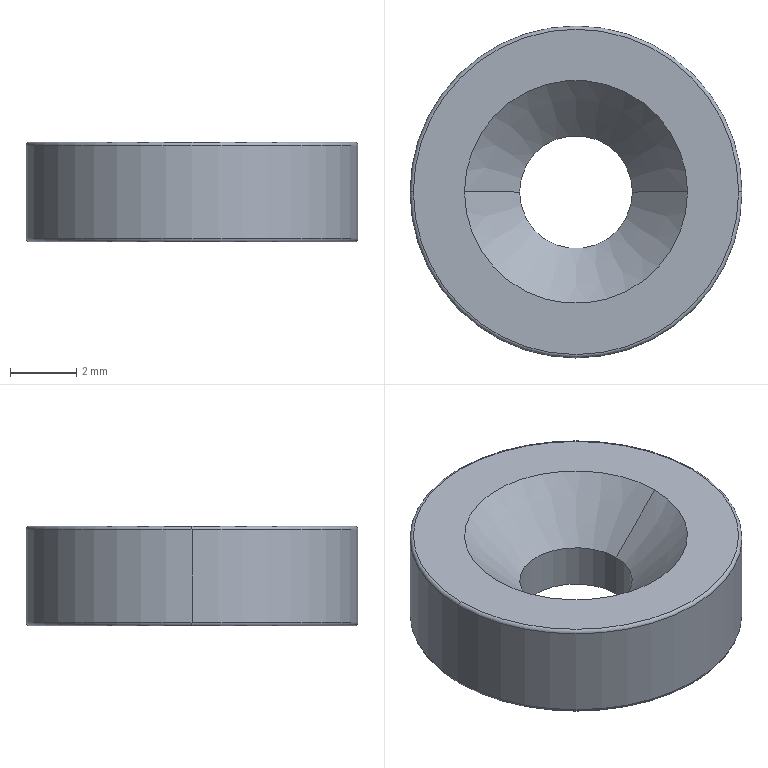Part | STEP file | QA-KZH10-3 | 1 solid | 12 faces | box 10 x 10 x 3 mm | volume 188.741 mm3 | torus 4 | cylinder 4 | cone 2 | plane 2 | commonest cylinder face diameters 3.4 x2 10 x2
STEP:
#1=CARTESIAN_POINT('',(0.,0.,0.));
#2=DIRECTION('',(0.,0.,1.));
#3=DIRECTION('',(1.,0.,0.));
#4=AXIS2_PLACEMENT_3D('',#1,#2,#3);
#5=CARTESIAN_POINT('',(-5.,0.,2.9));
#6=VERTEX_POINT('',#5);
#7=CARTESIAN_POINT('',(5.,0.,2.9));
#8=VERTEX_POINT('',#7);
#9=CARTESIAN_POINT('',(0.,0.,2.9));
#10=DIRECTION('',(0.,0.,-1.));
#11=DIRECTION('',(1.,0.,0.));
#12=AXIS2_PLACEMENT_3D('',#9,#10,#11);
#13=CIRCLE('',#12,5.);
#14=CARTESIAN_POINT('',(0.,0.,2.9));
#15=DIRECTION('',(0.,0.,1.));
#16=DIRECTION('',(1.,0.,0.));
#17=AXIS2_PLACEMENT_3D('',#14,#15,#16);
#18=TOROIDAL_SURFACE('',#17,4.9,0.1);
#19=CARTESIAN_POINT('',(6.283,0.));
#20=DIRECTION('',(-1.,0.));
#21=VECTOR('',#20,1.);
#22=LINE('',#19,#21);
#23=(GEOMETRIC_REPRESENTATION_CONTEXT(2)PARAMETRIC_REPRESENTATION_CONTEXT()REPRESENTATION_CONTEXT('',''));
#24=DEFINITIONAL_REPRESENTATION('',(#22),#23);
#25=PCURVE('',#18,#24);
#26=CARTESIAN_POINT('',(0.,0.,3.));
#27=DIRECTION('',(0.,0.,-1.));
#28=DIRECTION('',(-1.,0.,0.));
#29=AXIS2_PLACEMENT_3D('',#26,#27,#28);
#30=CYLINDRICAL_SURFACE('',#29,5.);
#31=CARTESIAN_POINT('',(-3.142,0.1));
#32=DIRECTION('',(1.,0.));
#33=VECTOR('',#32,1.);
#34=LINE('',#31,#33);
#35=(GEOMETRIC_REPRESENTATION_CONTEXT(2)PARAMETRIC_REPRESENTATION_CONTEXT()REPRESENTATION_CONTEXT('',''));
#36=DEFINITIONAL_REPRESENTATION('',(#34),#35);
#37=PCURVE('',#30,#36);
#38=SURFACE_CURVE('',#13,(#25,#37),.PCURVE_S1.);
#39=EDGE_CURVE('',#6,#8,#38,.T.);
#40=ORIENTED_EDGE('',*,*,#39,.F.);
#41=CARTESIAN_POINT('',(-4.9,0.,3.));
#42=VERTEX_POINT('',#41);
#43=CARTESIAN_POINT('',(-4.9,0.,2.9));
#44=DIRECTION('',(0.,1.,0.));
#45=DIRECTION('',(-1.,0.,0.));
#46=AXIS2_PLACEMENT_3D('',#43,#44,#45);
#47=CIRCLE('',#46,0.1);
#48=CARTESIAN_POINT('',(3.142,0.));
#49=DIRECTION('',(0.,1.));
#50=VECTOR('',#49,1.);
#51=LINE('',#48,#50);
#52=(GEOMETRIC_REPRESENTATION_CONTEXT(2)PARAMETRIC_REPRESENTATION_CONTEXT()REPRESENTATION_CONTEXT('',''));
#53=DEFINITIONAL_REPRESENTATION('',(#51),#52);
#54=PCURVE('',#18,#53);
#55=CARTESIAN_POINT('',(0.,0.,2.9));
#56=DIRECTION('',(0.,0.,1.));
#57=DIRECTION('',(1.,0.,0.));
#58=AXIS2_PLACEMENT_3D('',#55,#56,#57);
#59=TOROIDAL_SURFACE('',#58,4.9,0.1);
#60=CARTESIAN_POINT('',(3.142,0.));
#61=DIRECTION('',(0.,1.));
#62=VECTOR('',#61,1.);
#63=LINE('',#60,#62);
#64=(GEOMETRIC_REPRESENTATION_CONTEXT(2)PARAMETRIC_REPRESENTATION_CONTEXT()REPRESENTATION_CONTEXT('',''));
#65=DEFINITIONAL_REPRESENTATION('',(#63),#64);
#66=PCURVE('',#59,#65);
#67=SURFACE_CURVE('',#47,(#54,#66),.PCURVE_S1.);
#68=EDGE_CURVE('',#6,#42,#67,.T.);
#69=ORIENTED_EDGE('',*,*,#68,.T.);
#70=CARTESIAN_POINT('',(4.9,0.,3.));
#71=VERTEX_POINT('',#70);
#72=CARTESIAN_POINT('',(0.,0.,3.));
#73=DIRECTION('',(0.,0.,1.));
#74=DIRECTION('',(1.,0.,0.));
#75=AXIS2_PLACEMENT_3D('',#72,#73,#74);
#76=CIRCLE('',#75,4.9);
#77=CARTESIAN_POINT('',(0.,1.571));
#78=DIRECTION('',(1.,0.));
#79=VECTOR('',#78,1.);
#80=LINE('',#77,#79);
#81=(GEOMETRIC_REPRESENTATION_CONTEXT(2)PARAMETRIC_REPRESENTATION_CONTEXT()REPRESENTATION_CONTEXT('',''));
#82=DEFINITIONAL_REPRESENTATION('',(#80),#81);
#83=PCURVE('',#18,#82);
#84=CARTESIAN_POINT('',(0.,0.,3.));
#85=DIRECTION('',(0.,0.,1.));
#86=DIRECTION('',(1.,0.,0.));
#87=AXIS2_PLACEMENT_3D('',#84,#85,#86);
#88=PLANE('',#87);
#89=CARTESIAN_POINT('',(0.,0.));
#90=DIRECTION('',(1.,0.));
#91=AXIS2_PLACEMENT_2D('',#89,#90);
#92=CIRCLE('',#91,4.9);
#93=(GEOMETRIC_REPRESENTATION_CONTEXT(2)PARAMETRIC_REPRESENTATION_CONTEXT()REPRESENTATION_CONTEXT('',''));
#94=DEFINITIONAL_REPRESENTATION('',(#92),#93);
#95=PCURVE('',#88,#94);
#96=SURFACE_CURVE('',#76,(#83,#95),.PCURVE_S1.);
#97=EDGE_CURVE('',#71,#42,#96,.T.);
#98=ORIENTED_EDGE('',*,*,#97,.F.);
#99=CARTESIAN_POINT('',(4.9,0.,2.9));
#100=DIRECTION('',(0.,-1.,0.));
#101=DIRECTION('',(0.,0.,-1.));
#102=AXIS2_PLACEMENT_3D('',#99,#100,#101);
#103=CIRCLE('',#102,0.1);
#104=CARTESIAN_POINT('',(0.,-1.571));
#105=DIRECTION('',(0.,1.));
#106=VECTOR('',#105,1.);
#107=LINE('',#104,#106);
#108=(GEOMETRIC_REPRESENTATION_CONTEXT(2)PARAMETRIC_REPRESENTATION_CONTEXT()REPRESENTATION_CONTEXT('',''));
#109=DEFINITIONAL_REPRESENTATION('',(#107),#108);
#110=PCURVE('',#18,#109);
#111=CARTESIAN_POINT('',(6.283,-1.571));
#112=DIRECTION('',(0.,1.));
#113=VECTOR('',#112,1.);
#114=LINE('',#111,#113);
#115=(GEOMETRIC_REPRESENTATION_CONTEXT(2)PARAMETRIC_REPRESENTATION_CONTEXT()REPRESENTATION_CONTEXT('',''));
#116=DEFINITIONAL_REPRESENTATION('',(#114),#115);
#117=PCURVE('',#59,#116);
#118=SURFACE_CURVE('',#103,(#110,#117),.PCURVE_S1.);
#119=EDGE_CURVE('',#8,#71,#118,.T.);
#120=ORIENTED_EDGE('',*,*,#119,.F.);
#121=EDGE_LOOP('',(#40,#69,#98,#120));
#122=FACE_BOUND('',#121,.T.);
#123=ADVANCED_FACE('',(#122),#18,.T.);
#124=CARTESIAN_POINT('',(-4.9,0.,0.));
#125=VERTEX_POINT('',#124);
#126=CARTESIAN_POINT('',(4.9,0.,0.));
#127=VERTEX_POINT('',#126);
#128=CARTESIAN_POINT('',(0.,0.,0.));
#129=DIRECTION('',(0.,0.,-1.));
#130=DIRECTION('',(1.,0.,0.));
#131=AXIS2_PLACEMENT_3D('',#128,#129,#130);
#132=CIRCLE('',#131,4.9);
#133=CARTESIAN_POINT('',(0.,0.,0.1));
#134=DIRECTION('',(0.,0.,1.));
#135=DIRECTION('',(1.,0.,0.));
#136=AXIS2_PLACEMENT_3D('',#133,#134,#135);
#137=TOROIDAL_SURFACE('',#136,4.9,0.1);
#138=CARTESIAN_POINT('',(6.283,4.712));
#139=DIRECTION('',(-1.,0.));
#140=VECTOR('',#139,1.);
#141=LINE('',#138,#140);
#142=(GEOMETRIC_REPRESENTATION_CONTEXT(2)PARAMETRIC_REPRESENTATION_CONTEXT()REPRESENTATION_CONTEXT('',''));
#143=DEFINITIONAL_REPRESENTATION('',(#141),#142);
#144=PCURVE('',#137,#143);
#145=CARTESIAN_POINT('',(0.,0.,0.));
#146=DIRECTION('',(0.,0.,1.));
#147=DIRECTION('',(1.,0.,0.));
#148=AXIS2_PLACEMENT_3D('',#145,#146,#147);
#149=PLANE('',#148);
#150=CARTESIAN_POINT('',(4.9,0.));
#151=CARTESIAN_POINT('',(4.9,-8.487));
#152=CARTESIAN_POINT('',(-2.45,-4.244));
#153=CARTESIAN_POINT('',(-9.8,0.));
#154=CARTESIAN_POINT('',(-2.45,4.244));
#155=CARTESIAN_POINT('',(4.9,8.487));
#156=CARTESIAN_POINT('',(4.9,0.));
#157=(BOUNDED_CURVE()B_SPLINE_CURVE(2,(#150,#151,#152,#153,#154,#155,#156),.UNSPECIFIED.,.T.,.F.)B_SPLINE_CURVE_WITH_KNOTS((1,2,2,2,2,1),(-2.094,0.,2.094,4.189,6.283,8.378),.UNSPECIFIED.)CURVE()GEOMETRIC_REPRESENTATION_ITEM()RATIONAL_B_SPLINE_CURVE((1.,0.5,1.,0.5,1.,0.5,1.))REPRESENTATION_ITEM(''));
#158=(GEOMETRIC_REPRESENTATION_CONTEXT(2)PARAMETRIC_REPRESENTATION_CONTEXT()REPRESENTATION_CONTEXT('',''));
#159=DEFINITIONAL_REPRESENTATION('',(#157),#158);
#160=PCURVE('',#149,#159);
#161=SURFACE_CURVE('',#132,(#144,#160),.PCURVE_S1.);
#162=EDGE_CURVE('',#125,#127,#161,.T.);
#163=ORIENTED_EDGE('',*,*,#162,.F.);
#164=CARTESIAN_POINT('',(-5.,0.,0.1));
#165=VERTEX_POINT('',#164);
#166=CARTESIAN_POINT('',(-4.9,0.,0.1));
#167=DIRECTION('',(0.,1.,0.));
#168=DIRECTION('',(-1.,0.,0.));
#169=AXIS2_PLACEMENT_3D('',#166,#167,#168);
#170=CIRCLE('',#169,0.1);
#171=CARTESIAN_POINT('',(3.142,0.));
#172=DIRECTION('',(0.,1.));
#173=VECTOR('',#172,1.);
#174=LINE('',#171,#173);
#175=(GEOMETRIC_REPRESENTATION_CONTEXT(2)PARAMETRIC_REPRESENTATION_CONTEXT()REPRESENTATION_CONTEXT('',''));
#176=DEFINITIONAL_REPRESENTATION('',(#174),#175);
#177=PCURVE('',#137,#176);
#178=CARTESIAN_POINT('',(0.,0.,0.1));
#179=DIRECTION('',(0.,0.,1.));
#180=DIRECTION('',(1.,0.,0.));
#181=AXIS2_PLACEMENT_3D('',#178,#179,#180);
#182=TOROIDAL_SURFACE('',#181,4.9,0.1);
#183=CARTESIAN_POINT('',(3.142,0.));
#184=DIRECTION('',(0.,1.));
#185=VECTOR('',#184,1.);
#186=LINE('',#183,#185);
#187=(GEOMETRIC_REPRESENTATION_CONTEXT(2)PARAMETRIC_REPRESENTATION_CONTEXT()REPRESENTATION_CONTEXT('',''));
#188=DEFINITIONAL_REPRESENTATION('',(#186),#187);
#189=PCURVE('',#182,#188);
#190=SURFACE_CURVE('',#170,(#177,#189),.PCURVE_S1.);
#191=EDGE_CURVE('',#125,#165,#190,.T.);
#192=ORIENTED_EDGE('',*,*,#191,.T.);
#193=CARTESIAN_POINT('',(5.,0.,0.1));
#194=VERTEX_POINT('',#193);
#195=CARTESIAN_POINT('',(0.,0.,0.1));
#196=DIRECTION('',(0.,0.,1.));
#197=DIRECTION('',(1.,0.,0.));
#198=AXIS2_PLACEMENT_3D('',#195,#196,#197);
#199=CIRCLE('',#198,5.);
#200=CARTESIAN_POINT('',(0.,6.283));
#201=DIRECTION('',(1.,0.));
#202=VECTOR('',#201,1.);
#203=LINE('',#200,#202);
#204=(GEOMETRIC_REPRESENTATION_CONTEXT(2)PARAMETRIC_REPRESENTATION_CONTEXT()REPRESENTATION_CONTEXT('',''));
#205=DEFINITIONAL_REPRESENTATION('',(#203),#204);
#206=PCURVE('',#137,#205);
#207=CARTESIAN_POINT('',(3.142,2.9));
#208=DIRECTION('',(-1.,0.));
#209=VECTOR('',#208,1.);
#210=LINE('',#207,#209);
#211=(GEOMETRIC_REPRESENTATION_CONTEXT(2)PARAMETRIC_REPRESENTATION_CONTEXT()REPRESENTATION_CONTEXT('',''));
#212=DEFINITIONAL_REPRESENTATION('',(#210),#211);
#213=PCURVE('',#30,#212);
#214=SURFACE_CURVE('',#199,(#206,#213),.PCURVE_S1.);
#215=EDGE_CURVE('',#194,#165,#214,.T.);
#216=ORIENTED_EDGE('',*,*,#215,.F.);
#217=CARTESIAN_POINT('',(4.9,0.,0.1));
#218=DIRECTION('',(0.,-1.,0.));
#219=DIRECTION('',(0.,0.,-1.));
#220=AXIS2_PLACEMENT_3D('',#217,#218,#219);
#221=CIRCLE('',#220,0.1);
#222=CARTESIAN_POINT('',(0.,4.712));
#223=DIRECTION('',(0.,1.));
#224=VECTOR('',#223,1.);
#225=LINE('',#222,#224);
#226=(GEOMETRIC_REPRESENTATION_CONTEXT(2)PARAMETRIC_REPRESENTATION_CONTEXT()REPRESENTATION_CONTEXT('',''));
#227=DEFINITIONAL_REPRESENTATION('',(#225),#226);
#228=PCURVE('',#137,#227);
#229=CARTESIAN_POINT('',(6.283,4.712));
#230=DIRECTION('',(0.,1.));
#231=VECTOR('',#230,1.);
#232=LINE('',#229,#231);
#233=(GEOMETRIC_REPRESENTATION_CONTEXT(2)PARAMETRIC_REPRESENTATION_CONTEXT()REPRESENTATION_CONTEXT('',''));
#234=DEFINITIONAL_REPRESENTATION('',(#232),#233);
#235=PCURVE('',#182,#234);
#236=SURFACE_CURVE('',#221,(#228,#235),.PCURVE_S1.);
#237=EDGE_CURVE('',#127,#194,#236,.T.);
#238=ORIENTED_EDGE('',*,*,#237,.F.);
#239=EDGE_LOOP('',(#163,#192,#216,#238));
#240=FACE_BOUND('',#239,.T.);
#241=ADVANCED_FACE('',(#240),#137,.T.);
#242=CARTESIAN_POINT('',(1.7,0.,1.34));
#243=VERTEX_POINT('',#242);
#244=CARTESIAN_POINT('',(3.36,0.,3.));
#245=VERTEX_POINT('',#244);
#246=CARTESIAN_POINT('',(3.36,0.,3.));
#247=DIRECTION('',(0.7071,0.,0.7071));
#248=VECTOR('',#247,1.);
#249=LINE('',#246,#248);
#250=CARTESIAN_POINT('',(0.,0.,3.));
#251=DIRECTION('',(0.,0.,1.));
#252=DIRECTION('',(1.,0.,0.));
#253=AXIS2_PLACEMENT_3D('',#250,#251,#252);
#254=CONICAL_SURFACE('',#253,3.36,0.7854);
#255=CARTESIAN_POINT('',(6.283,0.));
#256=DIRECTION('',(0.,1.));
#257=VECTOR('',#256,1.);
#258=LINE('',#255,#257);
#259=(GEOMETRIC_REPRESENTATION_CONTEXT(2)PARAMETRIC_REPRESENTATION_CONTEXT()REPRESENTATION_CONTEXT('',''));
#260=DEFINITIONAL_REPRESENTATION('',(#258),#259);
#261=PCURVE('',#254,#260);
#262=CARTESIAN_POINT('',(0.,0.,3.));
#263=DIRECTION('',(0.,0.,1.));
#264=DIRECTION('',(1.,0.,0.));
#265=AXIS2_PLACEMENT_3D('',#262,#263,#264);
#266=CONICAL_SURFACE('',#265,3.36,0.7854);
#267=CARTESIAN_POINT('',(0.,0.));
#268=DIRECTION('',(0.,1.));
#269=VECTOR('',#268,1.);
#270=LINE('',#267,#269);
#271=(GEOMETRIC_REPRESENTATION_CONTEXT(2)PARAMETRIC_REPRESENTATION_CONTEXT()REPRESENTATION_CONTEXT('',''));
#272=DEFINITIONAL_REPRESENTATION('',(#270),#271);
#273=PCURVE('',#266,#272);
#274=SURFACE_CURVE('',#249,(#261,#273),.PCURVE_S1.);
#275=EDGE_CURVE('',#243,#245,#274,.T.);
#276=ORIENTED_EDGE('',*,*,#275,.T.);
#277=CARTESIAN_POINT('',(-3.36,0.,3.));
#278=VERTEX_POINT('',#277);
#279=CARTESIAN_POINT('',(0.,0.,3.));
#280=DIRECTION('',(0.,0.,1.));
#281=DIRECTION('',(1.,0.,0.));
#282=AXIS2_PLACEMENT_3D('',#279,#280,#281);
#283=CIRCLE('',#282,3.36);
#284=CARTESIAN_POINT('',(0.,0.));
#285=DIRECTION('',(1.,0.));
#286=VECTOR('',#285,1.);
#287=LINE('',#284,#286);
#288=(GEOMETRIC_REPRESENTATION_CONTEXT(2)PARAMETRIC_REPRESENTATION_CONTEXT()REPRESENTATION_CONTEXT('',''));
#289=DEFINITIONAL_REPRESENTATION('',(#287),#288);
#290=PCURVE('',#254,#289);
#291=CARTESIAN_POINT('',(0.,0.));
#292=DIRECTION('',(1.,0.));
#293=AXIS2_PLACEMENT_2D('',#291,#292);
#294=CIRCLE('',#293,3.36);
#295=(GEOMETRIC_REPRESENTATION_CONTEXT(2)PARAMETRIC_REPRESENTATION_CONTEXT()REPRESENTATION_CONTEXT('',''));
#296=DEFINITIONAL_REPRESENTATION('',(#294),#295);
#297=PCURVE('',#88,#296);
#298=SURFACE_CURVE('',#283,(#290,#297),.PCURVE_S1.);
#299=EDGE_CURVE('',#278,#245,#298,.T.);
#300=ORIENTED_EDGE('',*,*,#299,.F.);
#301=CARTESIAN_POINT('',(-1.7,0.,1.34));
#302=VERTEX_POINT('',#301);
#303=CARTESIAN_POINT('',(-3.36,0.,3.));
#304=DIRECTION('',(-0.7071,0.,0.7071));
#305=VECTOR('',#304,1.);
#306=LINE('',#303,#305);
#307=CARTESIAN_POINT('',(3.142,0.));
#308=DIRECTION('',(0.,1.));
#309=VECTOR('',#308,1.);
#310=LINE('',#307,#309);
#311=(GEOMETRIC_REPRESENTATION_CONTEXT(2)PARAMETRIC_REPRESENTATION_CONTEXT()REPRESENTATION_CONTEXT('',''));
#312=DEFINITIONAL_REPRESENTATION('',(#310),#311);
#313=PCURVE('',#254,#312);
#314=CARTESIAN_POINT('',(3.142,0.));
#315=DIRECTION('',(0.,1.));
#316=VECTOR('',#315,1.);
#317=LINE('',#314,#316);
#318=(GEOMETRIC_REPRESENTATION_CONTEXT(2)PARAMETRIC_REPRESENTATION_CONTEXT()REPRESENTATION_CONTEXT('',''));
#319=DEFINITIONAL_REPRESENTATION('',(#317),#318);
#320=PCURVE('',#266,#319);
#321=SURFACE_CURVE('',#306,(#313,#320),.PCURVE_S1.);
#322=EDGE_CURVE('',#302,#278,#321,.T.);
#323=ORIENTED_EDGE('',*,*,#322,.F.);
#324=CARTESIAN_POINT('',(0.,0.,1.34));
#325=DIRECTION('',(0.,0.,1.));
#326=DIRECTION('',(1.,0.,0.));
#327=AXIS2_PLACEMENT_3D('',#324,#325,#326);
#328=CIRCLE('',#327,1.7);
#329=CARTESIAN_POINT('',(0.,-1.66));
#330=DIRECTION('',(1.,0.));
#331=VECTOR('',#330,1.);
#332=LINE('',#329,#331);
#333=(GEOMETRIC_REPRESENTATION_CONTEXT(2)PARAMETRIC_REPRESENTATION_CONTEXT()REPRESENTATION_CONTEXT('',''));
#334=DEFINITIONAL_REPRESENTATION('',(#332),#333);
#335=PCURVE('',#254,#334);
#336=CARTESIAN_POINT('',(0.,0.,3.));
#337=DIRECTION('',(0.,0.,1.));
#338=DIRECTION('',(1.,0.,0.));
#339=AXIS2_PLACEMENT_3D('',#336,#337,#338);
#340=CYLINDRICAL_SURFACE('',#339,1.7);
#341=CARTESIAN_POINT('',(0.,-1.66));
#342=DIRECTION('',(1.,0.));
#343=VECTOR('',#342,1.);
#344=LINE('',#341,#343);
#345=(GEOMETRIC_REPRESENTATION_CONTEXT(2)PARAMETRIC_REPRESENTATION_CONTEXT()REPRESENTATION_CONTEXT('',''));
#346=DEFINITIONAL_REPRESENTATION('',(#344),#345);
#347=PCURVE('',#340,#346);
#348=SURFACE_CURVE('',#328,(#335,#347),.PCURVE_S1.);
#349=EDGE_CURVE('',#302,#243,#348,.T.);
#350=ORIENTED_EDGE('',*,*,#349,.T.);
#351=EDGE_LOOP('',(#276,#300,#323,#350));
#352=FACE_BOUND('',#351,.F.);
#353=ADVANCED_FACE('',(#352),#254,.F.);
#354=CARTESIAN_POINT('',(1.7,0.,0.));
#355=VERTEX_POINT('',#354);
#356=CARTESIAN_POINT('',(1.7,0.,3.));
#357=DIRECTION('',(0.,0.,1.));
#358=VECTOR('',#357,1.);
#359=LINE('',#356,#358);
#360=CARTESIAN_POINT('',(6.283,0.));
#361=DIRECTION('',(0.,1.));
#362=VECTOR('',#361,1.);
#363=LINE('',#360,#362);
#364=(GEOMETRIC_REPRESENTATION_CONTEXT(2)PARAMETRIC_REPRESENTATION_CONTEXT()REPRESENTATION_CONTEXT('',''));
#365=DEFINITIONAL_REPRESENTATION('',(#363),#364);
#366=PCURVE('',#340,#365);
#367=CARTESIAN_POINT('',(0.,0.,3.));
#368=DIRECTION('',(0.,0.,1.));
#369=DIRECTION('',(1.,0.,0.));
#370=AXIS2_PLACEMENT_3D('',#367,#368,#369);
#371=CYLINDRICAL_SURFACE('',#370,1.7);
#372=CARTESIAN_POINT('',(0.,0.));
#373=DIRECTION('',(0.,1.));
#374=VECTOR('',#373,1.);
#375=LINE('',#372,#374);
#376=(GEOMETRIC_REPRESENTATION_CONTEXT(2)PARAMETRIC_REPRESENTATION_CONTEXT()REPRESENTATION_CONTEXT('',''));
#377=DEFINITIONAL_REPRESENTATION('',(#375),#376);
#378=PCURVE('',#371,#377);
#379=SURFACE_CURVE('',#359,(#366,#378),.PCURVE_S1.);
#380=EDGE_CURVE('',#355,#243,#379,.T.);
#381=ORIENTED_EDGE('',*,*,#380,.T.);
#382=ORIENTED_EDGE('',*,*,#349,.F.);
#383=CARTESIAN_POINT('',(-1.7,0.,0.));
#384=VERTEX_POINT('',#383);
#385=CARTESIAN_POINT('',(-1.7,0.,3.));
#386=DIRECTION('',(0.,0.,1.));
#387=VECTOR('',#386,1.);
#388=LINE('',#385,#387);
#389=CARTESIAN_POINT('',(3.142,0.));
#390=DIRECTION('',(0.,1.));
#391=VECTOR('',#390,1.);
#392=LINE('',#389,#391);
#393=(GEOMETRIC_REPRESENTATION_CONTEXT(2)PARAMETRIC_REPRESENTATION_CONTEXT()REPRESENTATION_CONTEXT('',''));
#394=DEFINITIONAL_REPRESENTATION('',(#392),#393);
#395=PCURVE('',#340,#394);
#396=CARTESIAN_POINT('',(3.142,0.));
#397=DIRECTION('',(0.,1.));
#398=VECTOR('',#397,1.);
#399=LINE('',#396,#398);
#400=(GEOMETRIC_REPRESENTATION_CONTEXT(2)PARAMETRIC_REPRESENTATION_CONTEXT()REPRESENTATION_CONTEXT('',''));
#401=DEFINITIONAL_REPRESENTATION('',(#399),#400);
#402=PCURVE('',#371,#401);
#403=SURFACE_CURVE('',#388,(#395,#402),.PCURVE_S1.);
#404=EDGE_CURVE('',#384,#302,#403,.T.);
#405=ORIENTED_EDGE('',*,*,#404,.F.);
#406=CARTESIAN_POINT('',(0.,0.,0.));
#407=DIRECTION('',(0.,0.,1.));
#408=DIRECTION('',(1.,0.,0.));
#409=AXIS2_PLACEMENT_3D('',#406,#407,#408);
#410=CIRCLE('',#409,1.7);
#411=CARTESIAN_POINT('',(0.,-3.));
#412=DIRECTION('',(1.,0.));
#413=VECTOR('',#412,1.);
#414=LINE('',#411,#413);
#415=(GEOMETRIC_REPRESENTATION_CONTEXT(2)PARAMETRIC_REPRESENTATION_CONTEXT()REPRESENTATION_CONTEXT('',''));
#416=DEFINITIONAL_REPRESENTATION('',(#414),#415);
#417=PCURVE('',#340,#416);
#418=CARTESIAN_POINT('',(0.,0.));
#419=DIRECTION('',(1.,0.));
#420=AXIS2_PLACEMENT_2D('',#418,#419);
#421=CIRCLE('',#420,1.7);
#422=(GEOMETRIC_REPRESENTATION_CONTEXT(2)PARAMETRIC_REPRESENTATION_CONTEXT()REPRESENTATION_CONTEXT('',''));
#423=DEFINITIONAL_REPRESENTATION('',(#421),#422);
#424=PCURVE('',#149,#423);
#425=SURFACE_CURVE('',#410,(#417,#424),.PCURVE_S1.);
#426=EDGE_CURVE('',#384,#355,#425,.T.);
#427=ORIENTED_EDGE('',*,*,#426,.T.);
#428=EDGE_LOOP('',(#381,#382,#405,#427));
#429=FACE_BOUND('',#428,.F.);
#430=ADVANCED_FACE('',(#429),#340,.F.);
#431=ORIENTED_EDGE('',*,*,#39,.T.);
#432=CARTESIAN_POINT('',(5.,0.,3.));
#433=DIRECTION('',(0.,0.,-1.));
#434=VECTOR('',#433,1.);
#435=LINE('',#432,#434);
#436=CARTESIAN_POINT('',(3.142,0.));
#437=DIRECTION('',(0.,1.));
#438=VECTOR('',#437,1.);
#439=LINE('',#436,#438);
#440=(GEOMETRIC_REPRESENTATION_CONTEXT(2)PARAMETRIC_REPRESENTATION_CONTEXT()REPRESENTATION_CONTEXT('',''));
#441=DEFINITIONAL_REPRESENTATION('',(#439),#440);
#442=PCURVE('',#30,#441);
#443=CARTESIAN_POINT('',(0.,0.,3.));
#444=DIRECTION('',(0.,0.,-1.));
#445=DIRECTION('',(-1.,0.,0.));
#446=AXIS2_PLACEMENT_3D('',#443,#444,#445);
#447=CYLINDRICAL_SURFACE('',#446,5.);
#448=CARTESIAN_POINT('',(3.142,0.));
#449=DIRECTION('',(0.,1.));
#450=VECTOR('',#449,1.);
#451=LINE('',#448,#450);
#452=(GEOMETRIC_REPRESENTATION_CONTEXT(2)PARAMETRIC_REPRESENTATION_CONTEXT()REPRESENTATION_CONTEXT('',''));
#453=DEFINITIONAL_REPRESENTATION('',(#451),#452);
#454=PCURVE('',#447,#453);
#455=SURFACE_CURVE('',#435,(#442,#454),.PCURVE_S1.);
#456=EDGE_CURVE('',#8,#194,#455,.T.);
#457=ORIENTED_EDGE('',*,*,#456,.T.);
#458=ORIENTED_EDGE('',*,*,#215,.T.);
#459=CARTESIAN_POINT('',(-5.,0.,3.));
#460=DIRECTION('',(0.,0.,-1.));
#461=VECTOR('',#460,1.);
#462=LINE('',#459,#461);
#463=CARTESIAN_POINT('',(0.,0.));
#464=DIRECTION('',(0.,1.));
#465=VECTOR('',#464,1.);
#466=LINE('',#463,#465);
#467=(GEOMETRIC_REPRESENTATION_CONTEXT(2)PARAMETRIC_REPRESENTATION_CONTEXT()REPRESENTATION_CONTEXT('',''));
#468=DEFINITIONAL_REPRESENTATION('',(#466),#467);
#469=PCURVE('',#30,#468);
#470=CARTESIAN_POINT('',(6.283,0.));
#471=DIRECTION('',(0.,1.));
#472=VECTOR('',#471,1.);
#473=LINE('',#470,#472);
#474=(GEOMETRIC_REPRESENTATION_CONTEXT(2)PARAMETRIC_REPRESENTATION_CONTEXT()REPRESENTATION_CONTEXT('',''));
#475=DEFINITIONAL_REPRESENTATION('',(#473),#474);
#476=PCURVE('',#447,#475);
#477=SURFACE_CURVE('',#462,(#469,#476),.PCURVE_S1.);
#478=EDGE_CURVE('',#6,#165,#477,.T.);
#479=ORIENTED_EDGE('',*,*,#478,.F.);
#480=EDGE_LOOP('',(#431,#457,#458,#479));
#481=FACE_BOUND('',#480,.T.);
#482=ADVANCED_FACE('',(#481),#30,.T.);
#483=ORIENTED_EDGE('',*,*,#456,.F.);
#484=CARTESIAN_POINT('',(0.,0.,2.9));
#485=DIRECTION('',(0.,0.,-1.));
#486=DIRECTION('',(1.,0.,0.));
#487=AXIS2_PLACEMENT_3D('',#484,#485,#486);
#488=CIRCLE('',#487,5.);
#489=CARTESIAN_POINT('',(3.142,0.1));
#490=DIRECTION('',(1.,0.));
#491=VECTOR('',#490,1.);
#492=LINE('',#489,#491);
#493=(GEOMETRIC_REPRESENTATION_CONTEXT(2)PARAMETRIC_REPRESENTATION_CONTEXT()REPRESENTATION_CONTEXT('',''));
#494=DEFINITIONAL_REPRESENTATION('',(#492),#493);
#495=PCURVE('',#447,#494);
#496=CARTESIAN_POINT('',(6.283,0.));
#497=DIRECTION('',(-1.,0.));
#498=VECTOR('',#497,1.);
#499=LINE('',#496,#498);
#500=(GEOMETRIC_REPRESENTATION_CONTEXT(2)PARAMETRIC_REPRESENTATION_CONTEXT()REPRESENTATION_CONTEXT('',''));
#501=DEFINITIONAL_REPRESENTATION('',(#499),#500);
#502=PCURVE('',#59,#501);
#503=SURFACE_CURVE('',#488,(#495,#502),.PCURVE_S1.);
#504=EDGE_CURVE('',#8,#6,#503,.T.);
#505=ORIENTED_EDGE('',*,*,#504,.T.);
#506=ORIENTED_EDGE('',*,*,#478,.T.);
#507=CARTESIAN_POINT('',(0.,0.,0.1));
#508=DIRECTION('',(0.,0.,1.));
#509=DIRECTION('',(1.,0.,0.));
#510=AXIS2_PLACEMENT_3D('',#507,#508,#509);
#511=CIRCLE('',#510,5.);
#512=CARTESIAN_POINT('',(9.425,2.9));
#513=DIRECTION('',(-1.,0.));
#514=VECTOR('',#513,1.);
#515=LINE('',#512,#514);
#516=(GEOMETRIC_REPRESENTATION_CONTEXT(2)PARAMETRIC_REPRESENTATION_CONTEXT()REPRESENTATION_CONTEXT('',''));
#517=DEFINITIONAL_REPRESENTATION('',(#515),#516);
#518=PCURVE('',#447,#517);
#519=CARTESIAN_POINT('',(0.,6.283));
#520=DIRECTION('',(1.,0.));
#521=VECTOR('',#520,1.);
#522=LINE('',#519,#521);
#523=(GEOMETRIC_REPRESENTATION_CONTEXT(2)PARAMETRIC_REPRESENTATION_CONTEXT()REPRESENTATION_CONTEXT('',''));
#524=DEFINITIONAL_REPRESENTATION('',(#522),#523);
#525=PCURVE('',#182,#524);
#526=SURFACE_CURVE('',#511,(#518,#525),.PCURVE_S1.);
#527=EDGE_CURVE('',#165,#194,#526,.T.);
#528=ORIENTED_EDGE('',*,*,#527,.T.);
#529=EDGE_LOOP('',(#483,#505,#506,#528));
#530=FACE_BOUND('',#529,.T.);
#531=ADVANCED_FACE('',(#530),#447,.T.);
#532=ORIENTED_EDGE('',*,*,#97,.T.);
#533=CARTESIAN_POINT('',(0.,0.,3.));
#534=DIRECTION('',(0.,0.,1.));
#535=DIRECTION('',(1.,0.,0.));
#536=AXIS2_PLACEMENT_3D('',#533,#534,#535);
#537=CIRCLE('',#536,4.9);
#538=CARTESIAN_POINT('',(0.,0.));
#539=DIRECTION('',(1.,0.));
#540=AXIS2_PLACEMENT_2D('',#538,#539);
#541=CIRCLE('',#540,4.9);
#542=(GEOMETRIC_REPRESENTATION_CONTEXT(2)PARAMETRIC_REPRESENTATION_CONTEXT()REPRESENTATION_CONTEXT('',''));
#543=DEFINITIONAL_REPRESENTATION('',(#541),#542);
#544=PCURVE('',#88,#543);
#545=CARTESIAN_POINT('',(0.,1.571));
#546=DIRECTION('',(1.,0.));
#547=VECTOR('',#546,1.);
#548=LINE('',#545,#547);
#549=(GEOMETRIC_REPRESENTATION_CONTEXT(2)PARAMETRIC_REPRESENTATION_CONTEXT()REPRESENTATION_CONTEXT('',''));
#550=DEFINITIONAL_REPRESENTATION('',(#548),#549);
#551=PCURVE('',#59,#550);
#552=SURFACE_CURVE('',#537,(#544,#551),.PCURVE_S1.);
#553=EDGE_CURVE('',#42,#71,#552,.T.);
#554=ORIENTED_EDGE('',*,*,#553,.T.);
#555=EDGE_LOOP('',(#532,#554));
#556=FACE_BOUND('',#555,.T.);
#557=CARTESIAN_POINT('',(0.,0.,3.));
#558=DIRECTION('',(0.,0.,1.));
#559=DIRECTION('',(1.,0.,0.));
#560=AXIS2_PLACEMENT_3D('',#557,#558,#559);
#561=CIRCLE('',#560,3.36);
#562=CARTESIAN_POINT('',(0.,0.));
#563=DIRECTION('',(1.,0.));
#564=AXIS2_PLACEMENT_2D('',#562,#563);
#565=CIRCLE('',#564,3.36);
#566=(GEOMETRIC_REPRESENTATION_CONTEXT(2)PARAMETRIC_REPRESENTATION_CONTEXT()REPRESENTATION_CONTEXT('',''));
#567=DEFINITIONAL_REPRESENTATION('',(#565),#566);
#568=PCURVE('',#88,#567);
#569=CARTESIAN_POINT('',(0.,0.));
#570=DIRECTION('',(1.,0.));
#571=VECTOR('',#570,1.);
#572=LINE('',#569,#571);
#573=(GEOMETRIC_REPRESENTATION_CONTEXT(2)PARAMETRIC_REPRESENTATION_CONTEXT()REPRESENTATION_CONTEXT('',''));
#574=DEFINITIONAL_REPRESENTATION('',(#572),#573);
#575=PCURVE('',#266,#574);
#576=SURFACE_CURVE('',#561,(#568,#575),.PCURVE_S1.);
#577=EDGE_CURVE('',#245,#278,#576,.T.);
#578=ORIENTED_EDGE('',*,*,#577,.F.);
#579=ORIENTED_EDGE('',*,*,#299,.F.);
#580=EDGE_LOOP('',(#578,#579));
#581=FACE_BOUND('',#580,.T.);
#582=ADVANCED_FACE('',(#556,#581),#88,.T.);
#583=CARTESIAN_POINT('',(0.,0.,0.));
#584=DIRECTION('',(0.,0.,-1.));
#585=DIRECTION('',(1.,0.,0.));
#586=AXIS2_PLACEMENT_3D('',#583,#584,#585);
#587=CIRCLE('',#586,4.9);
#588=CARTESIAN_POINT('',(4.9,0.));
#589=CARTESIAN_POINT('',(4.9,-8.487));
#590=CARTESIAN_POINT('',(-2.45,-4.244));
#591=CARTESIAN_POINT('',(-9.8,0.));
#592=CARTESIAN_POINT('',(-2.45,4.244));
#593=CARTESIAN_POINT('',(4.9,8.487));
#594=CARTESIAN_POINT('',(4.9,0.));
#595=(BOUNDED_CURVE()B_SPLINE_CURVE(2,(#588,#589,#590,#591,#592,#593,#594),.UNSPECIFIED.,.T.,.F.)B_SPLINE_CURVE_WITH_KNOTS((1,2,2,2,2,1),(-2.094,0.,2.094,4.189,6.283,8.378),.UNSPECIFIED.)CURVE()GEOMETRIC_REPRESENTATION_ITEM()RATIONAL_B_SPLINE_CURVE((1.,0.5,1.,0.5,1.,0.5,1.))REPRESENTATION_ITEM(''));
#596=(GEOMETRIC_REPRESENTATION_CONTEXT(2)PARAMETRIC_REPRESENTATION_CONTEXT()REPRESENTATION_CONTEXT('',''));
#597=DEFINITIONAL_REPRESENTATION('',(#595),#596);
#598=PCURVE('',#149,#597);
#599=CARTESIAN_POINT('',(6.283,4.712));
#600=DIRECTION('',(-1.,0.));
#601=VECTOR('',#600,1.);
#602=LINE('',#599,#601);
#603=(GEOMETRIC_REPRESENTATION_CONTEXT(2)PARAMETRIC_REPRESENTATION_CONTEXT()REPRESENTATION_CONTEXT('',''));
#604=DEFINITIONAL_REPRESENTATION('',(#602),#603);
#605=PCURVE('',#182,#604);
#606=SURFACE_CURVE('',#587,(#598,#605),.PCURVE_S1.);
#607=EDGE_CURVE('',#127,#125,#606,.T.);
#608=ORIENTED_EDGE('',*,*,#607,.T.);
#609=ORIENTED_EDGE('',*,*,#162,.T.);
#610=EDGE_LOOP('',(#608,#609));
#611=FACE_BOUND('',#610,.T.);
#612=CARTESIAN_POINT('',(0.,0.,0.));
#613=DIRECTION('',(0.,0.,1.));
#614=DIRECTION('',(1.,0.,0.));
#615=AXIS2_PLACEMENT_3D('',#612,#613,#614);
#616=CIRCLE('',#615,1.7);
#617=CARTESIAN_POINT('',(0.,0.));
#618=DIRECTION('',(1.,0.));
#619=AXIS2_PLACEMENT_2D('',#617,#618);
#620=CIRCLE('',#619,1.7);
#621=(GEOMETRIC_REPRESENTATION_CONTEXT(2)PARAMETRIC_REPRESENTATION_CONTEXT()REPRESENTATION_CONTEXT('',''));
#622=DEFINITIONAL_REPRESENTATION('',(#620),#621);
#623=PCURVE('',#149,#622);
#624=CARTESIAN_POINT('',(0.,-3.));
#625=DIRECTION('',(1.,0.));
#626=VECTOR('',#625,1.);
#627=LINE('',#624,#626);
#628=(GEOMETRIC_REPRESENTATION_CONTEXT(2)PARAMETRIC_REPRESENTATION_CONTEXT()REPRESENTATION_CONTEXT('',''));
#629=DEFINITIONAL_REPRESENTATION('',(#627),#628);
#630=PCURVE('',#371,#629);
#631=SURFACE_CURVE('',#616,(#623,#630),.PCURVE_S1.);
#632=EDGE_CURVE('',#355,#384,#631,.T.);
#633=ORIENTED_EDGE('',*,*,#632,.T.);
#634=ORIENTED_EDGE('',*,*,#426,.T.);
#635=EDGE_LOOP('',(#633,#634));
#636=FACE_BOUND('',#635,.T.);
#637=ADVANCED_FACE('',(#611,#636),#149,.F.);
#638=CARTESIAN_POINT('',(0.,0.,1.34));
#639=DIRECTION('',(0.,0.,1.));
#640=DIRECTION('',(1.,0.,0.));
#641=AXIS2_PLACEMENT_3D('',#638,#639,#640);
#642=CIRCLE('',#641,1.7);
#643=CARTESIAN_POINT('',(0.,-1.66));
#644=DIRECTION('',(1.,0.));
#645=VECTOR('',#644,1.);
#646=LINE('',#643,#645);
#647=(GEOMETRIC_REPRESENTATION_CONTEXT(2)PARAMETRIC_REPRESENTATION_CONTEXT()REPRESENTATION_CONTEXT('',''));
#648=DEFINITIONAL_REPRESENTATION('',(#646),#647);
#649=PCURVE('',#371,#648);
#650=CARTESIAN_POINT('',(0.,-1.66));
#651=DIRECTION('',(1.,0.));
#652=VECTOR('',#651,1.);
#653=LINE('',#650,#652);
#654=(GEOMETRIC_REPRESENTATION_CONTEXT(2)PARAMETRIC_REPRESENTATION_CONTEXT()REPRESENTATION_CONTEXT('',''));
#655=DEFINITIONAL_REPRESENTATION('',(#653),#654);
#656=PCURVE('',#266,#655);
#657=SURFACE_CURVE('',#642,(#649,#656),.PCURVE_S1.);
#658=EDGE_CURVE('',#243,#302,#657,.T.);
#659=ORIENTED_EDGE('',*,*,#658,.F.);
#660=ORIENTED_EDGE('',*,*,#380,.F.);
#661=ORIENTED_EDGE('',*,*,#632,.T.);
#662=ORIENTED_EDGE('',*,*,#404,.T.);
#663=EDGE_LOOP('',(#659,#660,#661,#662));
#664=FACE_BOUND('',#663,.F.);
#665=ADVANCED_FACE('',(#664),#371,.F.);
#666=ORIENTED_EDGE('',*,*,#577,.F.);
#667=ORIENTED_EDGE('',*,*,#275,.F.);
#668=ORIENTED_EDGE('',*,*,#658,.T.);
#669=ORIENTED_EDGE('',*,*,#322,.T.);
#670=EDGE_LOOP('',(#666,#667,#668,#669));
#671=FACE_BOUND('',#670,.F.);
#672=ADVANCED_FACE('',(#671),#266,.F.);
#673=ORIENTED_EDGE('',*,*,#191,.F.);
#674=ORIENTED_EDGE('',*,*,#607,.F.);
#675=ORIENTED_EDGE('',*,*,#237,.T.);
#676=ORIENTED_EDGE('',*,*,#527,.F.);
#677=EDGE_LOOP('',(#673,#674,#675,#676));
#678=FACE_BOUND('',#677,.T.);
#679=ADVANCED_FACE('',(#678),#182,.T.);
#680=ORIENTED_EDGE('',*,*,#68,.F.);
#681=ORIENTED_EDGE('',*,*,#504,.F.);
#682=ORIENTED_EDGE('',*,*,#119,.T.);
#683=ORIENTED_EDGE('',*,*,#553,.F.);
#684=EDGE_LOOP('',(#680,#681,#682,#683));
#685=FACE_BOUND('',#684,.T.);
#686=ADVANCED_FACE('',(#685),#59,.T.);
#687=CLOSED_SHELL('',(#123,#241,#353,#430,#482,#531,#582,#637,#665,#672,#679,#686));
#688=MANIFOLD_SOLID_BREP('',#687);
#689=(LENGTH_UNIT()NAMED_UNIT(*)SI_UNIT(.MILLI.,.METRE.));
#690=UNCERTAINTY_MEASURE_WITH_UNIT(LENGTH_MEASURE(0.0000001),#689,'','');
#691=(NAMED_UNIT(*)PLANE_ANGLE_UNIT()SI_UNIT($,.RADIAN.));
#692=(NAMED_UNIT(*)SI_UNIT($,.STERADIAN.)SOLID_ANGLE_UNIT());
#693=(GEOMETRIC_REPRESENTATION_CONTEXT(3)GLOBAL_UNCERTAINTY_ASSIGNED_CONTEXT((#690))GLOBAL_UNIT_ASSIGNED_CONTEXT((#689,#691,#692))REPRESENTATION_CONTEXT('',''));
#694=ADVANCED_BREP_SHAPE_REPRESENTATION('',(#4,#688),#693);